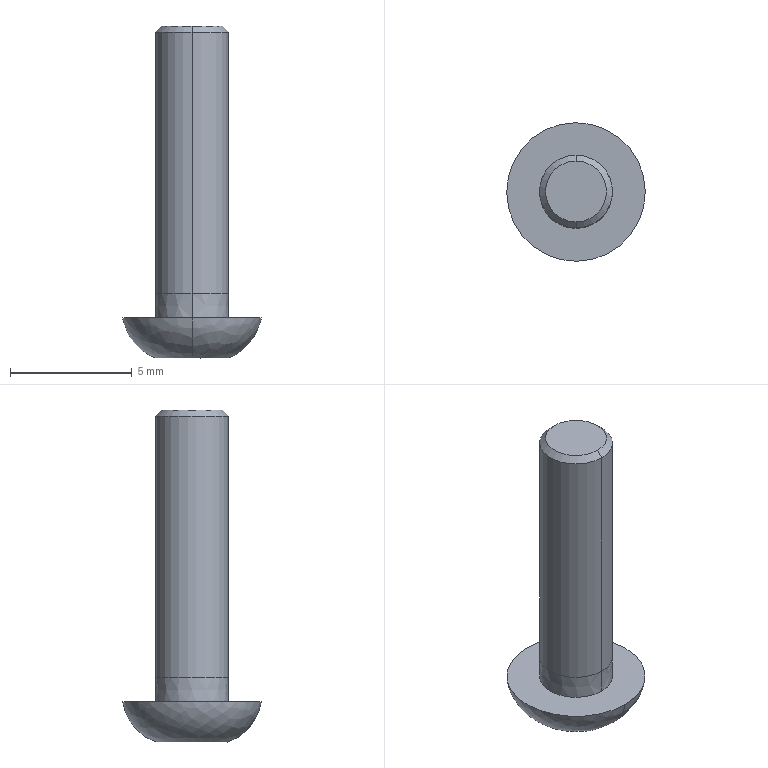Part | SolidWorks | features BaseBody 1 | 1 solid | 18 faces | box 5.7 x 5.7 x 13.65 mm | volume 112.119 mm3 | plane 10 | cone 4 | spline 2 | cylinder 2 | commonest cylinder face diameters 3 x2
STEP:
#1=CARTESIAN_POINT('',(689.526,-190.072,-85.234));
#2=VERTEX_POINT('',#1);
#3=CARTESIAN_POINT('',(689.502,-184.372,-85.234));
#4=VERTEX_POINT('',#3);
#5=CARTESIAN_POINT('',(689.514,-187.222,-85.234));
#6=DIRECTION('',(0.000000001,-0.000000003,1.));
#7=DIRECTION('',(0.,-1.,-0.000000003));
#8=AXIS2_PLACEMENT_3D('',#5,#6,#7);
#9=CIRCLE('',#8,2.85);
#10=EDGE_CURVE('',#2,#4,#9,.T.);
#11=ORIENTED_EDGE('',*,*,#10,.F.);
#12=CARTESIAN_POINT('',(689.521,-188.722,-86.884));
#13=VERTEX_POINT('',#12);
#14=CARTESIAN_POINT('',(689.517,-187.972,-84.893));
#15=DIRECTION('',(1.,0.004352,-0.000000001));
#16=DIRECTION('',(0.004352,-1.,-0.000000003));
#17=AXIS2_PLACEMENT_3D('',#14,#15,#16);
#18=CIRCLE('',#17,2.127);
#19=EDGE_CURVE('',#2,#13,#18,.T.);
#20=ORIENTED_EDGE('',*,*,#19,.T.);
#21=CARTESIAN_POINT('',(689.507,-185.722,-86.884));
#22=VERTEX_POINT('',#21);
#23=CARTESIAN_POINT('',(689.514,-187.222,-86.884));
#24=DIRECTION('',(0.000000001,-0.000000003,1.));
#25=DIRECTION('',(0.,-1.,-0.000000003));
#26=AXIS2_PLACEMENT_3D('',#23,#24,#25);
#27=CIRCLE('',#26,1.5);
#28=EDGE_CURVE('',#13,#22,#27,.T.);
#29=ORIENTED_EDGE('',*,*,#28,.T.);
#30=CARTESIAN_POINT('',(689.511,-186.472,-84.893));
#31=DIRECTION('',(-1.,-0.004352,0.000000001));
#32=DIRECTION('',(-0.004352,1.,0.000000003));
#33=AXIS2_PLACEMENT_3D('',#30,#31,#32);
#34=CIRCLE('',#33,2.127);
#35=EDGE_CURVE('',#4,#22,#34,.T.);
#36=ORIENTED_EDGE('',*,*,#35,.F.);
#37=EDGE_LOOP('',(#11,#20,#29,#36));
#38=FACE_OUTER_BOUND('',#37,.T.);
#39=CARTESIAN_POINT('',(689.526,-190.072,-85.234));
#40=CARTESIAN_POINT('',(695.226,-190.047,-85.234));
#41=CARTESIAN_POINT('',(695.202,-184.347,-85.234));
#42=CARTESIAN_POINT('',(689.502,-184.372,-85.234));
#43=CARTESIAN_POINT('',(689.526,-189.947,-86.005));
#44=CARTESIAN_POINT('',(694.976,-189.923,-86.005));
#45=CARTESIAN_POINT('',(694.952,-184.473,-86.005));
#46=CARTESIAN_POINT('',(689.502,-184.497,-86.005));
#47=CARTESIAN_POINT('',(689.524,-189.452,-86.609));
#48=CARTESIAN_POINT('',(693.985,-189.433,-86.609));
#49=CARTESIAN_POINT('',(693.965,-184.972,-86.609));
#50=CARTESIAN_POINT('',(689.504,-184.991,-86.609));
#51=CARTESIAN_POINT('',(689.521,-188.722,-86.884));
#52=CARTESIAN_POINT('',(692.521,-188.709,-86.884));
#53=CARTESIAN_POINT('',(692.507,-185.709,-86.884));
#54=CARTESIAN_POINT('',(689.507,-185.722,-86.884));
#55=(BOUNDED_SURFACE()B_SPLINE_SURFACE(3,3,((#39,#40,#41,#42),(#43,#44,#45,#46),(#47,#48,#49,#50),(#51,#52,#53,#54)),.UNSPECIFIED.,.F.,.F.,.T.)B_SPLINE_SURFACE_WITH_KNOTS((4,4),(4,4),(0.,1.),(0.,1.),.UNSPECIFIED.)GEOMETRIC_REPRESENTATION_ITEM()RATIONAL_B_SPLINE_SURFACE(((1.,0.3333,0.3333,1.),(0.9103,0.3034,0.3034,0.9103),(0.9103,0.3034,0.3034,0.9103),(1.,0.3333,0.3333,1.)))REPRESENTATION_ITEM('')SURFACE());
#56=ADVANCED_FACE('',(#38),#55,.T.);
#57=CARTESIAN_POINT('',(689.514,-188.722,-84.234));
#58=VERTEX_POINT('',#57);
#59=CARTESIAN_POINT('',(689.514,-185.722,-84.234));
#60=VERTEX_POINT('',#59);
#61=CARTESIAN_POINT('',(689.514,-187.222,-84.234));
#62=DIRECTION('',(0.000000001,-0.000000003,1.));
#63=DIRECTION('',(0.,-1.,-0.000000003));
#64=AXIS2_PLACEMENT_3D('',#61,#62,#63);
#65=CIRCLE('',#64,1.5);
#66=EDGE_CURVE('',#58,#60,#65,.T.);
#67=ORIENTED_EDGE('',*,*,#66,.T.);
#68=CARTESIAN_POINT('',(689.514,-185.722,-73.484));
#69=VERTEX_POINT('',#68);
#70=CARTESIAN_POINT('',(689.514,-185.722,-78.859));
#71=DIRECTION('',(0.000000001,-0.000000003,1.));
#72=VECTOR('',#71,1000.);
#73=LINE('',#70,#72);
#74=EDGE_CURVE('',#60,#69,#73,.T.);
#75=ORIENTED_EDGE('',*,*,#74,.T.);
#76=CARTESIAN_POINT('',(689.514,-188.722,-73.484));
#77=VERTEX_POINT('',#76);
#78=CARTESIAN_POINT('',(689.514,-187.222,-73.484));
#79=DIRECTION('',(-0.000000001,0.000000003,-1.));
#80=DIRECTION('',(0.,-1.,-0.000000003));
#81=AXIS2_PLACEMENT_3D('',#78,#79,#80);
#82=CIRCLE('',#81,1.5);
#83=EDGE_CURVE('',#69,#77,#82,.T.);
#84=ORIENTED_EDGE('',*,*,#83,.T.);
#85=CARTESIAN_POINT('',(689.514,-188.722,-78.859));
#86=DIRECTION('',(0.000000001,-0.000000003,1.));
#87=VECTOR('',#86,1000.);
#88=LINE('',#85,#87);
#89=EDGE_CURVE('',#58,#77,#88,.T.);
#90=ORIENTED_EDGE('',*,*,#89,.F.);
#91=EDGE_LOOP('',(#67,#75,#84,#90));
#92=FACE_OUTER_BOUND('',#91,.T.);
#93=CARTESIAN_POINT('',(689.514,-187.222,-78.859));
#94=DIRECTION('',(0.000000001,-0.000000003,1.));
#95=DIRECTION('',(0.,-1.,-0.000000003));
#96=AXIS2_PLACEMENT_3D('',#93,#94,#95);
#97=CYLINDRICAL_SURFACE('',#96,1.5);
#98=ADVANCED_FACE('',(#92),#97,.T.);
#99=CARTESIAN_POINT('',(689.514,-185.972,-73.234));
#100=VERTEX_POINT('',#99);
#101=CARTESIAN_POINT('',(689.514,-188.472,-73.234));
#102=VERTEX_POINT('',#101);
#103=CARTESIAN_POINT('',(689.514,-187.222,-73.234));
#104=DIRECTION('',(-0.000000001,0.000000003,-1.));
#105=DIRECTION('',(0.,1.,0.000000003));
#106=AXIS2_PLACEMENT_3D('',#103,#104,#105);
#107=CIRCLE('',#106,1.25);
#108=EDGE_CURVE('',#100,#102,#107,.T.);
#109=ORIENTED_EDGE('',*,*,#108,.T.);
#110=CARTESIAN_POINT('',(689.514,-188.722,-73.484));
#111=DIRECTION('',(-0.000000001,-0.7071,-0.7071));
#112=VECTOR('',#111,1000.);
#113=LINE('',#110,#112);
#114=EDGE_CURVE('',#102,#77,#113,.T.);
#115=ORIENTED_EDGE('',*,*,#114,.T.);
#116=ORIENTED_EDGE('',*,*,#83,.F.);
#117=CARTESIAN_POINT('',(689.514,-185.722,-73.484));
#118=DIRECTION('',(-0.000000001,0.7071,-0.7071));
#119=VECTOR('',#118,1000.);
#120=LINE('',#117,#119);
#121=EDGE_CURVE('',#100,#69,#120,.T.);
#122=ORIENTED_EDGE('',*,*,#121,.F.);
#123=EDGE_LOOP('',(#109,#115,#116,#122));
#124=FACE_OUTER_BOUND('',#123,.T.);
#125=CARTESIAN_POINT('',(689.514,-187.222,-73.484));
#126=DIRECTION('',(-0.000000001,0.000000003,-1.));
#127=DIRECTION('',(0.,1.,0.000000003));
#128=AXIS2_PLACEMENT_3D('',#125,#126,#127);
#129=CONICAL_SURFACE('',#128,1.5,0.7854);
#130=ADVANCED_FACE('',(#124),#129,.T.);
#131=CARTESIAN_POINT('',(689.514,-188.721,-85.234));
#132=VERTEX_POINT('',#131);
#133=CARTESIAN_POINT('',(689.514,-185.723,-85.234));
#134=VERTEX_POINT('',#133);
#135=CARTESIAN_POINT('',(689.514,-187.222,-85.234));
#136=DIRECTION('',(0.000000001,-0.000000003,1.));
#137=DIRECTION('',(0.,-1.,-0.000000003));
#138=AXIS2_PLACEMENT_3D('',#135,#136,#137);
#139=CIRCLE('',#138,1.499);
#140=EDGE_CURVE('',#132,#134,#139,.T.);
#141=ORIENTED_EDGE('',*,*,#140,.T.);
#142=CARTESIAN_POINT('',(689.514,-185.722,-84.234));
#143=DIRECTION('',(0.000000001,0.00075,1.));
#144=VECTOR('',#143,1000.);
#145=LINE('',#142,#144);
#146=EDGE_CURVE('',#134,#60,#145,.T.);
#147=ORIENTED_EDGE('',*,*,#146,.T.);
#148=ORIENTED_EDGE('',*,*,#66,.F.);
#149=CARTESIAN_POINT('',(689.514,-188.722,-84.234));
#150=DIRECTION('',(0.000000001,-0.00075,1.));
#151=VECTOR('',#150,1000.);
#152=LINE('',#149,#151);
#153=EDGE_CURVE('',#132,#58,#152,.T.);
#154=ORIENTED_EDGE('',*,*,#153,.F.);
#155=EDGE_LOOP('',(#141,#147,#148,#154));
#156=FACE_OUTER_BOUND('',#155,.T.);
#157=CARTESIAN_POINT('',(689.514,-187.222,-84.234));
#158=DIRECTION('',(0.000000001,-0.000000003,1.));
#159=DIRECTION('',(0.,-1.,-0.000000003));
#160=AXIS2_PLACEMENT_3D('',#157,#158,#159);
#161=CONICAL_SURFACE('',#160,1.5,0.00075);
#162=ADVANCED_FACE('',(#156),#161,.T.);
#163=ORIENTED_EDGE('',*,*,#74,.F.);
#164=CARTESIAN_POINT('',(689.514,-187.222,-84.234));
#165=DIRECTION('',(0.000000001,-0.000000003,1.));
#166=DIRECTION('',(0.,-1.,-0.000000003));
#167=AXIS2_PLACEMENT_3D('',#164,#165,#166);
#168=CIRCLE('',#167,1.5);
#169=EDGE_CURVE('',#60,#58,#168,.T.);
#170=ORIENTED_EDGE('',*,*,#169,.T.);
#171=ORIENTED_EDGE('',*,*,#89,.T.);
#172=CARTESIAN_POINT('',(689.514,-187.222,-73.484));
#173=DIRECTION('',(-0.000000001,0.000000003,-1.));
#174=DIRECTION('',(0.,-1.,-0.000000003));
#175=AXIS2_PLACEMENT_3D('',#172,#173,#174);
#176=CIRCLE('',#175,1.5);
#177=EDGE_CURVE('',#77,#69,#176,.T.);
#178=ORIENTED_EDGE('',*,*,#177,.T.);
#179=EDGE_LOOP('',(#163,#170,#171,#178));
#180=FACE_OUTER_BOUND('',#179,.T.);
#181=CARTESIAN_POINT('',(689.514,-187.222,-78.859));
#182=DIRECTION('',(0.000000001,-0.000000003,1.));
#183=DIRECTION('',(0.,-1.,-0.000000003));
#184=AXIS2_PLACEMENT_3D('',#181,#182,#183);
#185=CYLINDRICAL_SURFACE('',#184,1.5);
#186=ADVANCED_FACE('',(#180),#185,.T.);
#187=ORIENTED_EDGE('',*,*,#114,.F.);
#188=CARTESIAN_POINT('',(689.514,-187.222,-73.234));
#189=DIRECTION('',(-0.000000001,0.000000003,-1.));
#190=DIRECTION('',(0.,1.,0.000000003));
#191=AXIS2_PLACEMENT_3D('',#188,#189,#190);
#192=CIRCLE('',#191,1.25);
#193=EDGE_CURVE('',#102,#100,#192,.T.);
#194=ORIENTED_EDGE('',*,*,#193,.T.);
#195=ORIENTED_EDGE('',*,*,#121,.T.);
#196=ORIENTED_EDGE('',*,*,#177,.F.);
#197=EDGE_LOOP('',(#187,#194,#195,#196));
#198=FACE_OUTER_BOUND('',#197,.T.);
#199=CARTESIAN_POINT('',(689.514,-187.222,-73.484));
#200=DIRECTION('',(-0.000000001,0.000000003,-1.));
#201=DIRECTION('',(0.,1.,0.000000003));
#202=AXIS2_PLACEMENT_3D('',#199,#200,#201);
#203=CONICAL_SURFACE('',#202,1.5,0.7854);
#204=ADVANCED_FACE('',(#198),#203,.T.);
#205=ORIENTED_EDGE('',*,*,#146,.F.);
#206=CARTESIAN_POINT('',(689.514,-187.222,-85.234));
#207=DIRECTION('',(0.000000001,-0.000000003,1.));
#208=DIRECTION('',(0.,-1.,-0.000000003));
#209=AXIS2_PLACEMENT_3D('',#206,#207,#208);
#210=CIRCLE('',#209,1.499);
#211=EDGE_CURVE('',#134,#132,#210,.T.);
#212=ORIENTED_EDGE('',*,*,#211,.T.);
#213=ORIENTED_EDGE('',*,*,#153,.T.);
#214=ORIENTED_EDGE('',*,*,#169,.F.);
#215=EDGE_LOOP('',(#205,#212,#213,#214));
#216=FACE_OUTER_BOUND('',#215,.T.);
#217=CARTESIAN_POINT('',(689.514,-187.222,-84.234));
#218=DIRECTION('',(0.000000001,-0.000000003,1.));
#219=DIRECTION('',(0.,-1.,-0.000000003));
#220=AXIS2_PLACEMENT_3D('',#217,#218,#219);
#221=CONICAL_SURFACE('',#220,1.5,0.00075);
#222=ADVANCED_FACE('',(#216),#221,.T.);
#223=ORIENTED_EDGE('',*,*,#108,.F.);
#224=ORIENTED_EDGE('',*,*,#193,.F.);
#225=EDGE_LOOP('',(#223,#224));
#226=FACE_OUTER_BOUND('',#225,.T.);
#227=CARTESIAN_POINT('',(689.511,-186.597,-73.234));
#228=DIRECTION('',(0.000000001,-0.000000003,1.));
#229=DIRECTION('',(0.,-1.,-0.000000003));
#230=AXIS2_PLACEMENT_3D('',#227,#228,#229);
#231=PLANE('',#230);
#232=ADVANCED_FACE('',(#226),#231,.T.);
#233=ORIENTED_EDGE('',*,*,#140,.F.);
#234=ORIENTED_EDGE('',*,*,#211,.F.);
#235=EDGE_LOOP('',(#233,#234));
#236=FACE_BOUND('',#235,.T.);
#237=CARTESIAN_POINT('',(689.514,-187.222,-85.234));
#238=DIRECTION('',(0.000000001,-0.000000003,1.));
#239=DIRECTION('',(0.,-1.,-0.000000003));
#240=AXIS2_PLACEMENT_3D('',#237,#238,#239);
#241=CIRCLE('',#240,2.85);
#242=EDGE_CURVE('',#4,#2,#241,.T.);
#243=ORIENTED_EDGE('',*,*,#242,.T.);
#244=ORIENTED_EDGE('',*,*,#10,.T.);
#245=EDGE_LOOP('',(#243,#244));
#246=FACE_OUTER_BOUND('',#245,.T.);
#247=CARTESIAN_POINT('',(689.508,-185.797,-85.234));
#248=DIRECTION('',(0.000000001,-0.000000003,1.));
#249=DIRECTION('',(0.,-1.,-0.000000003));
#250=AXIS2_PLACEMENT_3D('',#247,#248,#249);
#251=PLANE('',#250);
#252=ADVANCED_FACE('',(#236,#246),#251,.T.);
#253=ORIENTED_EDGE('',*,*,#19,.F.);
#254=ORIENTED_EDGE('',*,*,#242,.F.);
#255=ORIENTED_EDGE('',*,*,#35,.T.);
#256=CARTESIAN_POINT('',(689.514,-187.222,-86.884));
#257=DIRECTION('',(0.000000001,-0.000000003,1.));
#258=DIRECTION('',(0.,-1.,-0.000000003));
#259=AXIS2_PLACEMENT_3D('',#256,#257,#258);
#260=CIRCLE('',#259,1.5);
#261=EDGE_CURVE('',#22,#13,#260,.T.);
#262=ORIENTED_EDGE('',*,*,#261,.T.);
#263=EDGE_LOOP('',(#253,#254,#255,#262));
#264=FACE_OUTER_BOUND('',#263,.T.);
#265=CARTESIAN_POINT('',(689.502,-184.372,-85.234));
#266=CARTESIAN_POINT('',(683.802,-184.397,-85.234));
#267=CARTESIAN_POINT('',(683.826,-190.097,-85.234));
#268=CARTESIAN_POINT('',(689.526,-190.072,-85.234));
#269=CARTESIAN_POINT('',(689.502,-184.497,-86.005));
#270=CARTESIAN_POINT('',(684.052,-184.521,-86.005));
#271=CARTESIAN_POINT('',(684.076,-189.97,-86.005));
#272=CARTESIAN_POINT('',(689.526,-189.947,-86.005));
#273=CARTESIAN_POINT('',(689.504,-184.991,-86.609));
#274=CARTESIAN_POINT('',(685.043,-185.011,-86.609));
#275=CARTESIAN_POINT('',(685.063,-189.472,-86.609));
#276=CARTESIAN_POINT('',(689.524,-189.452,-86.609));
#277=CARTESIAN_POINT('',(689.507,-185.722,-86.884));
#278=CARTESIAN_POINT('',(686.508,-185.735,-86.884));
#279=CARTESIAN_POINT('',(686.521,-188.735,-86.884));
#280=CARTESIAN_POINT('',(689.521,-188.722,-86.884));
#281=(BOUNDED_SURFACE()B_SPLINE_SURFACE(3,3,((#265,#266,#267,#268),(#269,#270,#271,#272),(#273,#274,#275,#276),(#277,#278,#279,#280)),.UNSPECIFIED.,.F.,.F.,.F.)B_SPLINE_SURFACE_WITH_KNOTS((4,4),(4,4),(0.,1.),(0.,1.),.UNSPECIFIED.)GEOMETRIC_REPRESENTATION_ITEM()RATIONAL_B_SPLINE_SURFACE(((1.,0.3333,0.3333,1.),(0.9103,0.3034,0.3034,0.9103),(0.9103,0.3034,0.3034,0.9103),(1.,0.3333,0.3333,1.)))REPRESENTATION_ITEM('')SURFACE());
#282=ADVANCED_FACE('',(#264),#281,.T.);
#283=ORIENTED_EDGE('',*,*,#261,.F.);
#284=ORIENTED_EDGE('',*,*,#28,.F.);
#285=EDGE_LOOP('',(#283,#284));
#286=FACE_OUTER_BOUND('',#285,.T.);
#287=CARTESIAN_POINT('',(688.517,-187.803,-86.884));
#288=VERTEX_POINT('',#287);
#289=CARTESIAN_POINT('',(689.519,-188.376,-86.884));
#290=VERTEX_POINT('',#289);
#291=CARTESIAN_POINT('',(688.517,-187.803,-86.884));
#292=DIRECTION('',(0.8682,-0.4962,-0.000000002));
#293=VECTOR('',#292,1000.);
#294=LINE('',#291,#293);
#295=EDGE_CURVE('',#288,#290,#294,.T.);
#296=ORIENTED_EDGE('',*,*,#295,.T.);
#297=CARTESIAN_POINT('',(690.517,-187.795,-86.884));
#298=VERTEX_POINT('',#297);
#299=CARTESIAN_POINT('',(689.519,-188.376,-86.884));
#300=DIRECTION('',(0.8638,0.5038,0.000000001));
#301=VECTOR('',#300,1000.);
#302=LINE('',#299,#301);
#303=EDGE_CURVE('',#290,#298,#302,.T.);
#304=ORIENTED_EDGE('',*,*,#303,.T.);
#305=CARTESIAN_POINT('',(690.511,-186.64,-86.884));
#306=VERTEX_POINT('',#305);
#307=CARTESIAN_POINT('',(690.517,-187.795,-86.884));
#308=DIRECTION('',(-0.004352,1.,0.000000003));
#309=VECTOR('',#308,1000.);
#310=LINE('',#307,#309);
#311=EDGE_CURVE('',#298,#306,#310,.T.);
#312=ORIENTED_EDGE('',*,*,#311,.T.);
#313=CARTESIAN_POINT('',(689.509,-186.067,-86.884));
#314=VERTEX_POINT('',#313);
#315=CARTESIAN_POINT('',(690.511,-186.64,-86.884));
#316=DIRECTION('',(-0.8682,0.4962,0.000000002));
#317=VECTOR('',#316,1000.);
#318=LINE('',#315,#317);
#319=EDGE_CURVE('',#306,#314,#318,.T.);
#320=ORIENTED_EDGE('',*,*,#319,.T.);
#321=CARTESIAN_POINT('',(688.512,-186.649,-86.884));
#322=VERTEX_POINT('',#321);
#323=CARTESIAN_POINT('',(689.509,-186.067,-86.884));
#324=DIRECTION('',(-0.8638,-0.5038,-0.000000001));
#325=VECTOR('',#324,1000.);
#326=LINE('',#323,#325);
#327=EDGE_CURVE('',#314,#322,#326,.T.);
#328=ORIENTED_EDGE('',*,*,#327,.T.);
#329=CARTESIAN_POINT('',(688.512,-186.649,-86.884));
#330=DIRECTION('',(0.004352,-1.,-0.000000003));
#331=VECTOR('',#330,1000.);
#332=LINE('',#329,#331);
#333=EDGE_CURVE('',#322,#288,#332,.T.);
#334=ORIENTED_EDGE('',*,*,#333,.T.);
#335=EDGE_LOOP('',(#296,#304,#312,#320,#328,#334));
#336=FACE_BOUND('',#335,.T.);
#337=CARTESIAN_POINT('',(689.511,-186.472,-86.884));
#338=DIRECTION('',(-0.000000001,0.000000003,-1.));
#339=DIRECTION('',(0.,1.,0.000000003));
#340=AXIS2_PLACEMENT_3D('',#337,#338,#339);
#341=PLANE('',#340);
#342=ADVANCED_FACE('',(#286,#336),#341,.T.);
#343=CARTESIAN_POINT('',(690.517,-187.795,-85.844));
#344=VERTEX_POINT('',#343);
#345=CARTESIAN_POINT('',(690.517,-187.795,-86.884));
#346=DIRECTION('',(0.000000002,-0.000000003,1.));
#347=VECTOR('',#346,1000.);
#348=LINE('',#345,#347);
#349=EDGE_CURVE('',#298,#344,#348,.T.);
#350=ORIENTED_EDGE('',*,*,#349,.F.);
#351=ORIENTED_EDGE('',*,*,#303,.F.);
#352=CARTESIAN_POINT('',(689.519,-188.376,-85.844));
#353=VERTEX_POINT('',#352);
#354=CARTESIAN_POINT('',(689.519,-188.376,-86.884));
#355=DIRECTION('',(-0.000000002,0.000000003,-1.));
#356=VECTOR('',#355,1000.);
#357=LINE('',#354,#356);
#358=EDGE_CURVE('',#353,#290,#357,.T.);
#359=ORIENTED_EDGE('',*,*,#358,.F.);
#360=CARTESIAN_POINT('',(690.517,-187.795,-85.844));
#361=DIRECTION('',(-0.8638,-0.5038,0.));
#362=VECTOR('',#361,1000.);
#363=LINE('',#360,#362);
#364=EDGE_CURVE('',#344,#353,#363,.T.);
#365=ORIENTED_EDGE('',*,*,#364,.F.);
#366=EDGE_LOOP('',(#350,#351,#359,#365));
#367=FACE_OUTER_BOUND('',#366,.T.);
#368=CARTESIAN_POINT('',(690.517,-187.795,-86.884));
#369=DIRECTION('',(0.5038,-0.8638,-0.000000003));
#370=DIRECTION('',(0.8638,0.5038,0.));
#371=AXIS2_PLACEMENT_3D('',#368,#369,#370);
#372=PLANE('',#371);
#373=ADVANCED_FACE('',(#367),#372,.F.);
#374=ORIENTED_EDGE('',*,*,#358,.T.);
#375=ORIENTED_EDGE('',*,*,#295,.F.);
#376=CARTESIAN_POINT('',(688.517,-187.803,-85.844));
#377=VERTEX_POINT('',#376);
#378=CARTESIAN_POINT('',(688.517,-187.803,-86.884));
#379=DIRECTION('',(0.000000001,0.000000002,-1.));
#380=VECTOR('',#379,1000.);
#381=LINE('',#378,#380);
#382=EDGE_CURVE('',#377,#288,#381,.T.);
#383=ORIENTED_EDGE('',*,*,#382,.F.);
#384=CARTESIAN_POINT('',(689.519,-188.376,-85.844));
#385=DIRECTION('',(-0.8682,0.4962,0.));
#386=VECTOR('',#385,1000.);
#387=LINE('',#384,#386);
#388=EDGE_CURVE('',#353,#377,#387,.T.);
#389=ORIENTED_EDGE('',*,*,#388,.F.);
#390=EDGE_LOOP('',(#374,#375,#383,#389));
#391=FACE_OUTER_BOUND('',#390,.T.);
#392=CARTESIAN_POINT('',(689.519,-188.376,-86.884));
#393=DIRECTION('',(-0.4962,-0.8682,-0.000000003));
#394=DIRECTION('',(0.8682,-0.4962,0.));
#395=AXIS2_PLACEMENT_3D('',#392,#393,#394);
#396=PLANE('',#395);
#397=ADVANCED_FACE('',(#391),#396,.F.);
#398=ORIENTED_EDGE('',*,*,#382,.T.);
#399=ORIENTED_EDGE('',*,*,#333,.F.);
#400=CARTESIAN_POINT('',(688.512,-186.649,-85.844));
#401=VERTEX_POINT('',#400);
#402=CARTESIAN_POINT('',(688.512,-186.649,-86.884));
#403=DIRECTION('',(-0.000000001,0.,-1.));
#404=VECTOR('',#403,1000.);
#405=LINE('',#402,#404);
#406=EDGE_CURVE('',#401,#322,#405,.T.);
#407=ORIENTED_EDGE('',*,*,#406,.F.);
#408=CARTESIAN_POINT('',(688.517,-187.803,-85.844));
#409=DIRECTION('',(-0.004352,1.,0.));
#410=VECTOR('',#409,1000.);
#411=LINE('',#408,#410);
#412=EDGE_CURVE('',#377,#401,#411,.T.);
#413=ORIENTED_EDGE('',*,*,#412,.F.);
#414=EDGE_LOOP('',(#398,#399,#407,#413));
#415=FACE_OUTER_BOUND('',#414,.T.);
#416=CARTESIAN_POINT('',(688.517,-187.803,-86.884));
#417=DIRECTION('',(-1.,-0.004352,0.000000001));
#418=DIRECTION('',(0.004352,-1.,0.));
#419=AXIS2_PLACEMENT_3D('',#416,#417,#418);
#420=PLANE('',#419);
#421=ADVANCED_FACE('',(#415),#420,.F.);
#422=ORIENTED_EDGE('',*,*,#406,.T.);
#423=ORIENTED_EDGE('',*,*,#327,.F.);
#424=CARTESIAN_POINT('',(689.509,-186.067,-85.844));
#425=VERTEX_POINT('',#424);
#426=CARTESIAN_POINT('',(689.509,-186.067,-86.884));
#427=DIRECTION('',(-0.000000002,0.000000003,-1.));
#428=VECTOR('',#427,1000.);
#429=LINE('',#426,#428);
#430=EDGE_CURVE('',#425,#314,#429,.T.);
#431=ORIENTED_EDGE('',*,*,#430,.F.);
#432=CARTESIAN_POINT('',(688.512,-186.649,-85.844));
#433=DIRECTION('',(0.8638,0.5038,0.));
#434=VECTOR('',#433,1000.);
#435=LINE('',#432,#434);
#436=EDGE_CURVE('',#401,#425,#435,.T.);
#437=ORIENTED_EDGE('',*,*,#436,.F.);
#438=EDGE_LOOP('',(#422,#423,#431,#437));
#439=FACE_OUTER_BOUND('',#438,.T.);
#440=CARTESIAN_POINT('',(688.512,-186.649,-86.884));
#441=DIRECTION('',(-0.5038,0.8638,0.000000003));
#442=DIRECTION('',(-0.8638,-0.5038,0.));
#443=AXIS2_PLACEMENT_3D('',#440,#441,#442);
#444=PLANE('',#443);
#445=ADVANCED_FACE('',(#439),#444,.F.);
#446=ORIENTED_EDGE('',*,*,#430,.T.);
#447=ORIENTED_EDGE('',*,*,#319,.F.);
#448=CARTESIAN_POINT('',(690.511,-186.64,-85.844));
#449=VERTEX_POINT('',#448);
#450=CARTESIAN_POINT('',(690.511,-186.64,-86.884));
#451=DIRECTION('',(0.000000001,0.000000002,-1.));
#452=VECTOR('',#451,1000.);
#453=LINE('',#450,#452);
#454=EDGE_CURVE('',#449,#306,#453,.T.);
#455=ORIENTED_EDGE('',*,*,#454,.F.);
#456=CARTESIAN_POINT('',(689.509,-186.067,-85.844));
#457=DIRECTION('',(0.8682,-0.4962,0.));
#458=VECTOR('',#457,1000.);
#459=LINE('',#456,#458);
#460=EDGE_CURVE('',#425,#449,#459,.T.);
#461=ORIENTED_EDGE('',*,*,#460,.F.);
#462=EDGE_LOOP('',(#446,#447,#455,#461));
#463=FACE_OUTER_BOUND('',#462,.T.);
#464=CARTESIAN_POINT('',(689.509,-186.067,-86.884));
#465=DIRECTION('',(0.4962,0.8682,0.000000003));
#466=DIRECTION('',(-0.8682,0.4962,0.));
#467=AXIS2_PLACEMENT_3D('',#464,#465,#466);
#468=PLANE('',#467);
#469=ADVANCED_FACE('',(#463),#468,.F.);
#470=ORIENTED_EDGE('',*,*,#454,.T.);
#471=ORIENTED_EDGE('',*,*,#311,.F.);
#472=ORIENTED_EDGE('',*,*,#349,.T.);
#473=CARTESIAN_POINT('',(690.511,-186.64,-85.844));
#474=DIRECTION('',(0.004352,-1.,0.));
#475=VECTOR('',#474,1000.);
#476=LINE('',#473,#475);
#477=EDGE_CURVE('',#449,#344,#476,.T.);
#478=ORIENTED_EDGE('',*,*,#477,.F.);
#479=EDGE_LOOP('',(#470,#471,#472,#478));
#480=FACE_OUTER_BOUND('',#479,.T.);
#481=CARTESIAN_POINT('',(690.511,-186.64,-86.884));
#482=DIRECTION('',(1.,0.004352,-0.000000001));
#483=DIRECTION('',(-0.004352,1.,0.));
#484=AXIS2_PLACEMENT_3D('',#481,#482,#483);
#485=PLANE('',#484);
#486=ADVANCED_FACE('',(#480),#485,.F.);
#487=ORIENTED_EDGE('',*,*,#436,.T.);
#488=ORIENTED_EDGE('',*,*,#460,.T.);
#489=ORIENTED_EDGE('',*,*,#477,.T.);
#490=ORIENTED_EDGE('',*,*,#364,.T.);
#491=ORIENTED_EDGE('',*,*,#388,.T.);
#492=ORIENTED_EDGE('',*,*,#412,.T.);
#493=EDGE_LOOP('',(#487,#488,#489,#490,#491,#492));
#494=FACE_OUTER_BOUND('',#493,.T.);
#495=CARTESIAN_POINT('',(689.514,-187.222,-85.844));
#496=DIRECTION('',(-0.000000001,0.000000003,-1.));
#497=DIRECTION('',(0.,1.,0.000000003));
#498=AXIS2_PLACEMENT_3D('',#495,#496,#497);
#499=PLANE('',#498);
#500=ADVANCED_FACE('',(#494),#499,.T.);
#501=CLOSED_SHELL('',(#56,#98,#130,#162,#186,#204,#222,#232,#252,#282,#342,#373,#397,#421,#445,#469,#486,#500));
#502=MANIFOLD_SOLID_BREP('',#501);
#503=CARTESIAN_POINT('',(0.,0.,0.));
#504=DIRECTION('',(0.,0.,1.));
#505=DIRECTION('',(1.,0.,0.));
#506=AXIS2_PLACEMENT_3D('',#503,#504,#505);
#507=(LENGTH_UNIT()NAMED_UNIT(*)SI_UNIT(.MILLI.,.METRE.));
#508=UNCERTAINTY_MEASURE_WITH_UNIT(LENGTH_MEASURE(0.00001),#507,'','');
#509=(NAMED_UNIT(*)PLANE_ANGLE_UNIT()SI_UNIT($,.RADIAN.));
#510=(NAMED_UNIT(*)SI_UNIT($,.STERADIAN.)SOLID_ANGLE_UNIT());
#511=(GEOMETRIC_REPRESENTATION_CONTEXT(3)GLOBAL_UNCERTAINTY_ASSIGNED_CONTEXT((#508))GLOBAL_UNIT_ASSIGNED_CONTEXT((#507,#509,#510))REPRESENTATION_CONTEXT('',''));
#512=ADVANCED_BREP_SHAPE_REPRESENTATION('',(#502,#506),#511);